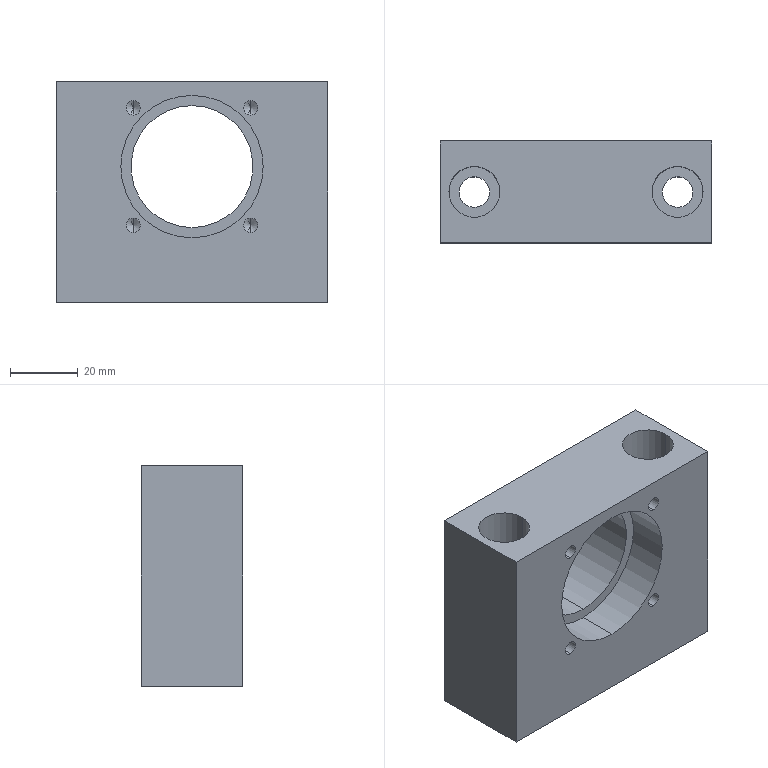Part | SolidWorks | features ICE 5, HoleWzd 4, Chamfer 1, Extrusion 1 | 1 solid | 37 faces | box 80 x 30 x 65 mm | volume 99631 mm3 | cylinder 20 | plane 9 | cone 8 | commonest cylinder face diameters 4.2 x8 9 x4 15 x4 36 x2 42 x2
STEP:
#1=CARTESIAN_POINT('',(17.324,-2.6,-7.724));
#2=VERTEX_POINT('',#1);
#3=CARTESIAN_POINT('',(17.324,-2.6,-11.924));
#4=VERTEX_POINT('',#3);
#5=CARTESIAN_POINT('',(17.324,-2.6,-9.824));
#6=DIRECTION('',(0.,-1.,0.));
#7=DIRECTION('',(0.,0.,-1.));
#8=AXIS2_PLACEMENT_3D('',#5,#6,#7);
#9=CIRCLE('',#8,2.1);
#10=EDGE_CURVE('',#2,#4,#9,.T.);
#11=ORIENTED_EDGE('',*,*,#10,.F.);
#12=CARTESIAN_POINT('',(17.324,-15.,-7.724));
#13=VERTEX_POINT('',#12);
#14=CARTESIAN_POINT('',(17.324,-15.,-7.724));
#15=DIRECTION('',(0.,-1.,0.));
#16=VECTOR('',#15,1000.);
#17=LINE('',#14,#16);
#18=EDGE_CURVE('',#2,#13,#17,.T.);
#19=ORIENTED_EDGE('',*,*,#18,.T.);
#20=CARTESIAN_POINT('',(17.324,-15.,-11.924));
#21=VERTEX_POINT('',#20);
#22=CARTESIAN_POINT('',(17.324,-15.,-9.824));
#23=DIRECTION('',(0.,-1.,0.));
#24=DIRECTION('',(0.,0.,-1.));
#25=AXIS2_PLACEMENT_3D('',#22,#23,#24);
#26=CIRCLE('',#25,2.1);
#27=EDGE_CURVE('',#13,#21,#26,.T.);
#28=ORIENTED_EDGE('',*,*,#27,.T.);
#29=CARTESIAN_POINT('',(17.324,-15.,-11.924));
#30=DIRECTION('',(0.,-1.,0.));
#31=VECTOR('',#30,1000.);
#32=LINE('',#29,#31);
#33=EDGE_CURVE('',#4,#21,#32,.T.);
#34=ORIENTED_EDGE('',*,*,#33,.F.);
#35=EDGE_LOOP('',(#11,#19,#28,#34));
#36=FACE_OUTER_BOUND('',#35,.T.);
#37=CARTESIAN_POINT('',(17.324,-15.,-9.824));
#38=DIRECTION('',(0.,-1.,0.));
#39=DIRECTION('',(0.,0.,-1.));
#40=AXIS2_PLACEMENT_3D('',#37,#38,#39);
#41=CYLINDRICAL_SURFACE('',#40,2.1);
#42=ADVANCED_FACE('',(#36),#41,.F.);
#43=CARTESIAN_POINT('',(17.324,-1.338,-9.824));
#44=VERTEX_POINT('',#43);
#45=CARTESIAN_POINT('',(17.324,-2.6,-11.924));
#46=DIRECTION('',(0.,-0.515,-0.8572));
#47=VECTOR('',#46,1000.);
#48=LINE('',#45,#47);
#49=EDGE_CURVE('',#44,#4,#48,.T.);
#50=ORIENTED_EDGE('',*,*,#49,.F.);
#51=CARTESIAN_POINT('',(17.324,-2.6,-7.724));
#52=DIRECTION('',(0.,-0.515,0.8572));
#53=VECTOR('',#52,1000.);
#54=LINE('',#51,#53);
#55=EDGE_CURVE('',#44,#2,#54,.T.);
#56=ORIENTED_EDGE('',*,*,#55,.T.);
#57=ORIENTED_EDGE('',*,*,#10,.T.);
#58=EDGE_LOOP('',(#50,#56,#57));
#59=FACE_OUTER_BOUND('',#58,.T.);
#60=CARTESIAN_POINT('',(17.324,-2.6,-9.824));
#61=DIRECTION('',(0.,-1.,0.));
#62=DIRECTION('',(0.,0.,-1.));
#63=AXIS2_PLACEMENT_3D('',#60,#61,#62);
#64=CONICAL_SURFACE('',#63,2.1,1.03);
#65=ADVANCED_FACE('',(#59),#64,.F.);
#66=CARTESIAN_POINT('',(-17.324,-2.6,-7.724));
#67=VERTEX_POINT('',#66);
#68=CARTESIAN_POINT('',(-17.324,-2.6,-11.924));
#69=VERTEX_POINT('',#68);
#70=CARTESIAN_POINT('',(-17.324,-2.6,-9.824));
#71=DIRECTION('',(0.,-1.,0.));
#72=DIRECTION('',(0.,0.,-1.));
#73=AXIS2_PLACEMENT_3D('',#70,#71,#72);
#74=CIRCLE('',#73,2.1);
#75=EDGE_CURVE('',#67,#69,#74,.T.);
#76=ORIENTED_EDGE('',*,*,#75,.F.);
#77=CARTESIAN_POINT('',(-17.324,-15.,-7.724));
#78=VERTEX_POINT('',#77);
#79=CARTESIAN_POINT('',(-17.324,-15.,-7.724));
#80=DIRECTION('',(0.,-1.,0.));
#81=VECTOR('',#80,1000.);
#82=LINE('',#79,#81);
#83=EDGE_CURVE('',#67,#78,#82,.T.);
#84=ORIENTED_EDGE('',*,*,#83,.T.);
#85=CARTESIAN_POINT('',(-17.324,-15.,-11.924));
#86=VERTEX_POINT('',#85);
#87=CARTESIAN_POINT('',(-17.324,-15.,-9.824));
#88=DIRECTION('',(0.,-1.,0.));
#89=DIRECTION('',(0.,0.,-1.));
#90=AXIS2_PLACEMENT_3D('',#87,#88,#89);
#91=CIRCLE('',#90,2.1);
#92=EDGE_CURVE('',#78,#86,#91,.T.);
#93=ORIENTED_EDGE('',*,*,#92,.T.);
#94=CARTESIAN_POINT('',(-17.324,-15.,-11.924));
#95=DIRECTION('',(0.,-1.,0.));
#96=VECTOR('',#95,1000.);
#97=LINE('',#94,#96);
#98=EDGE_CURVE('',#69,#86,#97,.T.);
#99=ORIENTED_EDGE('',*,*,#98,.F.);
#100=EDGE_LOOP('',(#76,#84,#93,#99));
#101=FACE_OUTER_BOUND('',#100,.T.);
#102=CARTESIAN_POINT('',(-17.324,-15.,-9.824));
#103=DIRECTION('',(0.,-1.,0.));
#104=DIRECTION('',(0.,0.,-1.));
#105=AXIS2_PLACEMENT_3D('',#102,#103,#104);
#106=CYLINDRICAL_SURFACE('',#105,2.1);
#107=ADVANCED_FACE('',(#101),#106,.F.);
#108=CARTESIAN_POINT('',(-17.324,-1.338,-9.824));
#109=VERTEX_POINT('',#108);
#110=CARTESIAN_POINT('',(-17.324,-2.6,-11.924));
#111=DIRECTION('',(0.,-0.515,-0.8572));
#112=VECTOR('',#111,1000.);
#113=LINE('',#110,#112);
#114=EDGE_CURVE('',#109,#69,#113,.T.);
#115=ORIENTED_EDGE('',*,*,#114,.F.);
#116=CARTESIAN_POINT('',(-17.324,-2.6,-7.724));
#117=DIRECTION('',(0.,-0.515,0.8572));
#118=VECTOR('',#117,1000.);
#119=LINE('',#116,#118);
#120=EDGE_CURVE('',#109,#67,#119,.T.);
#121=ORIENTED_EDGE('',*,*,#120,.T.);
#122=ORIENTED_EDGE('',*,*,#75,.T.);
#123=EDGE_LOOP('',(#115,#121,#122));
#124=FACE_OUTER_BOUND('',#123,.T.);
#125=CARTESIAN_POINT('',(-17.324,-2.6,-9.824));
#126=DIRECTION('',(0.,-1.,0.));
#127=DIRECTION('',(0.,0.,-1.));
#128=AXIS2_PLACEMENT_3D('',#125,#126,#127);
#129=CONICAL_SURFACE('',#128,2.1,1.03);
#130=ADVANCED_FACE('',(#124),#129,.F.);
#131=CARTESIAN_POINT('',(-17.324,-2.6,26.924));
#132=VERTEX_POINT('',#131);
#133=CARTESIAN_POINT('',(-17.324,-2.6,22.724));
#134=VERTEX_POINT('',#133);
#135=CARTESIAN_POINT('',(-17.324,-2.6,24.824));
#136=DIRECTION('',(0.,-1.,0.));
#137=DIRECTION('',(0.,0.,-1.));
#138=AXIS2_PLACEMENT_3D('',#135,#136,#137);
#139=CIRCLE('',#138,2.1);
#140=EDGE_CURVE('',#132,#134,#139,.T.);
#141=ORIENTED_EDGE('',*,*,#140,.F.);
#142=CARTESIAN_POINT('',(-17.324,-15.,26.924));
#143=VERTEX_POINT('',#142);
#144=CARTESIAN_POINT('',(-17.324,-15.,26.924));
#145=DIRECTION('',(0.,-1.,0.));
#146=VECTOR('',#145,1000.);
#147=LINE('',#144,#146);
#148=EDGE_CURVE('',#132,#143,#147,.T.);
#149=ORIENTED_EDGE('',*,*,#148,.T.);
#150=CARTESIAN_POINT('',(-17.324,-15.,22.724));
#151=VERTEX_POINT('',#150);
#152=CARTESIAN_POINT('',(-17.324,-15.,24.824));
#153=DIRECTION('',(0.,-1.,0.));
#154=DIRECTION('',(0.,0.,-1.));
#155=AXIS2_PLACEMENT_3D('',#152,#153,#154);
#156=CIRCLE('',#155,2.1);
#157=EDGE_CURVE('',#143,#151,#156,.T.);
#158=ORIENTED_EDGE('',*,*,#157,.T.);
#159=CARTESIAN_POINT('',(-17.324,-15.,22.724));
#160=DIRECTION('',(0.,-1.,0.));
#161=VECTOR('',#160,1000.);
#162=LINE('',#159,#161);
#163=EDGE_CURVE('',#134,#151,#162,.T.);
#164=ORIENTED_EDGE('',*,*,#163,.F.);
#165=EDGE_LOOP('',(#141,#149,#158,#164));
#166=FACE_OUTER_BOUND('',#165,.T.);
#167=CARTESIAN_POINT('',(-17.324,-15.,24.824));
#168=DIRECTION('',(0.,-1.,0.));
#169=DIRECTION('',(0.,0.,-1.));
#170=AXIS2_PLACEMENT_3D('',#167,#168,#169);
#171=CYLINDRICAL_SURFACE('',#170,2.1);
#172=ADVANCED_FACE('',(#166),#171,.F.);
#173=CARTESIAN_POINT('',(-17.324,-1.338,24.824));
#174=VERTEX_POINT('',#173);
#175=CARTESIAN_POINT('',(-17.324,-2.6,22.724));
#176=DIRECTION('',(0.,-0.515,-0.8572));
#177=VECTOR('',#176,1000.);
#178=LINE('',#175,#177);
#179=EDGE_CURVE('',#174,#134,#178,.T.);
#180=ORIENTED_EDGE('',*,*,#179,.F.);
#181=CARTESIAN_POINT('',(-17.324,-2.6,26.924));
#182=DIRECTION('',(0.,-0.515,0.8572));
#183=VECTOR('',#182,1000.);
#184=LINE('',#181,#183);
#185=EDGE_CURVE('',#174,#132,#184,.T.);
#186=ORIENTED_EDGE('',*,*,#185,.T.);
#187=ORIENTED_EDGE('',*,*,#140,.T.);
#188=EDGE_LOOP('',(#180,#186,#187));
#189=FACE_OUTER_BOUND('',#188,.T.);
#190=CARTESIAN_POINT('',(-17.324,-2.6,24.824));
#191=DIRECTION('',(0.,-1.,0.));
#192=DIRECTION('',(0.,0.,-1.));
#193=AXIS2_PLACEMENT_3D('',#190,#191,#192);
#194=CONICAL_SURFACE('',#193,2.1,1.03);
#195=ADVANCED_FACE('',(#189),#194,.F.);
#196=CARTESIAN_POINT('',(17.324,-2.6,26.924));
#197=VERTEX_POINT('',#196);
#198=CARTESIAN_POINT('',(17.324,-2.6,22.724));
#199=VERTEX_POINT('',#198);
#200=CARTESIAN_POINT('',(17.324,-2.6,24.824));
#201=DIRECTION('',(0.,-1.,0.));
#202=DIRECTION('',(0.,0.,-1.));
#203=AXIS2_PLACEMENT_3D('',#200,#201,#202);
#204=CIRCLE('',#203,2.1);
#205=EDGE_CURVE('',#197,#199,#204,.T.);
#206=ORIENTED_EDGE('',*,*,#205,.F.);
#207=CARTESIAN_POINT('',(17.324,-15.,26.924));
#208=VERTEX_POINT('',#207);
#209=CARTESIAN_POINT('',(17.324,-15.,26.924));
#210=DIRECTION('',(0.,-1.,0.));
#211=VECTOR('',#210,1000.);
#212=LINE('',#209,#211);
#213=EDGE_CURVE('',#197,#208,#212,.T.);
#214=ORIENTED_EDGE('',*,*,#213,.T.);
#215=CARTESIAN_POINT('',(17.324,-15.,22.724));
#216=VERTEX_POINT('',#215);
#217=CARTESIAN_POINT('',(17.324,-15.,24.824));
#218=DIRECTION('',(0.,-1.,0.));
#219=DIRECTION('',(0.,0.,-1.));
#220=AXIS2_PLACEMENT_3D('',#217,#218,#219);
#221=CIRCLE('',#220,2.1);
#222=EDGE_CURVE('',#208,#216,#221,.T.);
#223=ORIENTED_EDGE('',*,*,#222,.T.);
#224=CARTESIAN_POINT('',(17.324,-15.,22.724));
#225=DIRECTION('',(0.,-1.,0.));
#226=VECTOR('',#225,1000.);
#227=LINE('',#224,#226);
#228=EDGE_CURVE('',#199,#216,#227,.T.);
#229=ORIENTED_EDGE('',*,*,#228,.F.);
#230=EDGE_LOOP('',(#206,#214,#223,#229));
#231=FACE_OUTER_BOUND('',#230,.T.);
#232=CARTESIAN_POINT('',(17.324,-15.,24.824));
#233=DIRECTION('',(0.,-1.,0.));
#234=DIRECTION('',(0.,0.,-1.));
#235=AXIS2_PLACEMENT_3D('',#232,#233,#234);
#236=CYLINDRICAL_SURFACE('',#235,2.1);
#237=ADVANCED_FACE('',(#231),#236,.F.);
#238=CARTESIAN_POINT('',(17.324,-1.338,24.824));
#239=VERTEX_POINT('',#238);
#240=CARTESIAN_POINT('',(17.324,-2.6,22.724));
#241=DIRECTION('',(0.,-0.515,-0.8572));
#242=VECTOR('',#241,1000.);
#243=LINE('',#240,#242);
#244=EDGE_CURVE('',#239,#199,#243,.T.);
#245=ORIENTED_EDGE('',*,*,#244,.F.);
#246=CARTESIAN_POINT('',(17.324,-2.6,26.924));
#247=DIRECTION('',(0.,-0.515,0.8572));
#248=VECTOR('',#247,1000.);
#249=LINE('',#246,#248);
#250=EDGE_CURVE('',#239,#197,#249,.T.);
#251=ORIENTED_EDGE('',*,*,#250,.T.);
#252=ORIENTED_EDGE('',*,*,#205,.T.);
#253=EDGE_LOOP('',(#245,#251,#252));
#254=FACE_OUTER_BOUND('',#253,.T.);
#255=CARTESIAN_POINT('',(17.324,-2.6,24.824));
#256=DIRECTION('',(0.,-1.,0.));
#257=DIRECTION('',(0.,0.,-1.));
#258=AXIS2_PLACEMENT_3D('',#255,#256,#257);
#259=CONICAL_SURFACE('',#258,2.1,1.03);
#260=ADVANCED_FACE('',(#254),#259,.F.);
#261=CARTESIAN_POINT('',(22.5,0.,-22.5));
#262=VERTEX_POINT('',#261);
#263=CARTESIAN_POINT('',(37.5,0.,-22.5));
#264=VERTEX_POINT('',#263);
#265=CARTESIAN_POINT('',(30.,0.,-22.5));
#266=DIRECTION('',(0.,0.,1.));
#267=DIRECTION('',(1.,0.,0.));
#268=AXIS2_PLACEMENT_3D('',#265,#266,#267);
#269=CIRCLE('',#268,7.5);
#270=EDGE_CURVE('',#262,#264,#269,.T.);
#271=ORIENTED_EDGE('',*,*,#270,.F.);
#272=CARTESIAN_POINT('',(22.5,0.,32.5));
#273=VERTEX_POINT('',#272);
#274=CARTESIAN_POINT('',(22.5,0.,32.5));
#275=DIRECTION('',(0.,0.,1.));
#276=VECTOR('',#275,1000.);
#277=LINE('',#274,#276);
#278=EDGE_CURVE('',#262,#273,#277,.T.);
#279=ORIENTED_EDGE('',*,*,#278,.T.);
#280=CARTESIAN_POINT('',(37.5,0.,32.5));
#281=VERTEX_POINT('',#280);
#282=CARTESIAN_POINT('',(30.,0.,32.5));
#283=DIRECTION('',(0.,0.,1.));
#284=DIRECTION('',(1.,0.,0.));
#285=AXIS2_PLACEMENT_3D('',#282,#283,#284);
#286=CIRCLE('',#285,7.5);
#287=EDGE_CURVE('',#273,#281,#286,.T.);
#288=ORIENTED_EDGE('',*,*,#287,.T.);
#289=CARTESIAN_POINT('',(37.5,0.,32.5));
#290=DIRECTION('',(0.,0.,1.));
#291=VECTOR('',#290,1000.);
#292=LINE('',#289,#291);
#293=EDGE_CURVE('',#264,#281,#292,.T.);
#294=ORIENTED_EDGE('',*,*,#293,.F.);
#295=EDGE_LOOP('',(#271,#279,#288,#294));
#296=FACE_OUTER_BOUND('',#295,.T.);
#297=CARTESIAN_POINT('',(30.,0.,32.5));
#298=DIRECTION('',(0.,0.,1.));
#299=DIRECTION('',(1.,0.,0.));
#300=AXIS2_PLACEMENT_3D('',#297,#298,#299);
#301=CYLINDRICAL_SURFACE('',#300,7.5);
#302=ADVANCED_FACE('',(#296),#301,.F.);
#303=CARTESIAN_POINT('',(25.5,0.,-32.5));
#304=VERTEX_POINT('',#303);
#305=CARTESIAN_POINT('',(34.5,0.,-32.5));
#306=VERTEX_POINT('',#305);
#307=CARTESIAN_POINT('',(30.,0.,-32.5));
#308=DIRECTION('',(0.,0.,1.));
#309=DIRECTION('',(1.,0.,0.));
#310=AXIS2_PLACEMENT_3D('',#307,#308,#309);
#311=CIRCLE('',#310,4.5);
#312=EDGE_CURVE('',#304,#306,#311,.T.);
#313=ORIENTED_EDGE('',*,*,#312,.F.);
#314=CARTESIAN_POINT('',(25.5,0.,-22.5));
#315=VERTEX_POINT('',#314);
#316=CARTESIAN_POINT('',(25.5,0.,32.5));
#317=DIRECTION('',(0.,0.,1.));
#318=VECTOR('',#317,1000.);
#319=LINE('',#316,#318);
#320=EDGE_CURVE('',#304,#315,#319,.T.);
#321=ORIENTED_EDGE('',*,*,#320,.T.);
#322=CARTESIAN_POINT('',(34.5,0.,-22.5));
#323=VERTEX_POINT('',#322);
#324=CARTESIAN_POINT('',(30.,0.,-22.5));
#325=DIRECTION('',(0.,0.,1.));
#326=DIRECTION('',(1.,0.,0.));
#327=AXIS2_PLACEMENT_3D('',#324,#325,#326);
#328=CIRCLE('',#327,4.5);
#329=EDGE_CURVE('',#315,#323,#328,.T.);
#330=ORIENTED_EDGE('',*,*,#329,.T.);
#331=CARTESIAN_POINT('',(34.5,0.,32.5));
#332=DIRECTION('',(0.,0.,1.));
#333=VECTOR('',#332,1000.);
#334=LINE('',#331,#333);
#335=EDGE_CURVE('',#306,#323,#334,.T.);
#336=ORIENTED_EDGE('',*,*,#335,.F.);
#337=EDGE_LOOP('',(#313,#321,#330,#336));
#338=FACE_OUTER_BOUND('',#337,.T.);
#339=CARTESIAN_POINT('',(30.,0.,32.5));
#340=DIRECTION('',(0.,0.,1.));
#341=DIRECTION('',(1.,0.,0.));
#342=AXIS2_PLACEMENT_3D('',#339,#340,#341);
#343=CYLINDRICAL_SURFACE('',#342,4.5);
#344=ADVANCED_FACE('',(#338),#343,.F.);
#345=CARTESIAN_POINT('',(-37.5,0.,-22.5));
#346=VERTEX_POINT('',#345);
#347=CARTESIAN_POINT('',(-22.5,0.,-22.5));
#348=VERTEX_POINT('',#347);
#349=CARTESIAN_POINT('',(-30.,0.,-22.5));
#350=DIRECTION('',(0.,0.,1.));
#351=DIRECTION('',(1.,0.,0.));
#352=AXIS2_PLACEMENT_3D('',#349,#350,#351);
#353=CIRCLE('',#352,7.5);
#354=EDGE_CURVE('',#346,#348,#353,.T.);
#355=ORIENTED_EDGE('',*,*,#354,.F.);
#356=CARTESIAN_POINT('',(-37.5,0.,32.5));
#357=VERTEX_POINT('',#356);
#358=CARTESIAN_POINT('',(-37.5,0.,32.5));
#359=DIRECTION('',(0.,0.,1.));
#360=VECTOR('',#359,1000.);
#361=LINE('',#358,#360);
#362=EDGE_CURVE('',#346,#357,#361,.T.);
#363=ORIENTED_EDGE('',*,*,#362,.T.);
#364=CARTESIAN_POINT('',(-22.5,0.,32.5));
#365=VERTEX_POINT('',#364);
#366=CARTESIAN_POINT('',(-30.,0.,32.5));
#367=DIRECTION('',(0.,0.,1.));
#368=DIRECTION('',(1.,0.,0.));
#369=AXIS2_PLACEMENT_3D('',#366,#367,#368);
#370=CIRCLE('',#369,7.5);
#371=EDGE_CURVE('',#357,#365,#370,.T.);
#372=ORIENTED_EDGE('',*,*,#371,.T.);
#373=CARTESIAN_POINT('',(-22.5,0.,32.5));
#374=DIRECTION('',(0.,0.,1.));
#375=VECTOR('',#374,1000.);
#376=LINE('',#373,#375);
#377=EDGE_CURVE('',#348,#365,#376,.T.);
#378=ORIENTED_EDGE('',*,*,#377,.F.);
#379=EDGE_LOOP('',(#355,#363,#372,#378));
#380=FACE_OUTER_BOUND('',#379,.T.);
#381=CARTESIAN_POINT('',(-30.,0.,32.5));
#382=DIRECTION('',(0.,0.,1.));
#383=DIRECTION('',(1.,0.,0.));
#384=AXIS2_PLACEMENT_3D('',#381,#382,#383);
#385=CYLINDRICAL_SURFACE('',#384,7.5);
#386=ADVANCED_FACE('',(#380),#385,.F.);
#387=CARTESIAN_POINT('',(-34.5,0.,-32.5));
#388=VERTEX_POINT('',#387);
#389=CARTESIAN_POINT('',(-25.5,0.,-32.5));
#390=VERTEX_POINT('',#389);
#391=CARTESIAN_POINT('',(-30.,0.,-32.5));
#392=DIRECTION('',(0.,0.,1.));
#393=DIRECTION('',(1.,0.,0.));
#394=AXIS2_PLACEMENT_3D('',#391,#392,#393);
#395=CIRCLE('',#394,4.5);
#396=EDGE_CURVE('',#388,#390,#395,.T.);
#397=ORIENTED_EDGE('',*,*,#396,.F.);
#398=CARTESIAN_POINT('',(-34.5,0.,-22.5));
#399=VERTEX_POINT('',#398);
#400=CARTESIAN_POINT('',(-34.5,0.,32.5));
#401=DIRECTION('',(0.,0.,1.));
#402=VECTOR('',#401,1000.);
#403=LINE('',#400,#402);
#404=EDGE_CURVE('',#388,#399,#403,.T.);
#405=ORIENTED_EDGE('',*,*,#404,.T.);
#406=CARTESIAN_POINT('',(-25.5,0.,-22.5));
#407=VERTEX_POINT('',#406);
#408=CARTESIAN_POINT('',(-30.,0.,-22.5));
#409=DIRECTION('',(0.,0.,1.));
#410=DIRECTION('',(1.,0.,0.));
#411=AXIS2_PLACEMENT_3D('',#408,#409,#410);
#412=CIRCLE('',#411,4.5);
#413=EDGE_CURVE('',#399,#407,#412,.T.);
#414=ORIENTED_EDGE('',*,*,#413,.T.);
#415=CARTESIAN_POINT('',(-25.5,0.,32.5));
#416=DIRECTION('',(0.,0.,1.));
#417=VECTOR('',#416,1000.);
#418=LINE('',#415,#417);
#419=EDGE_CURVE('',#390,#407,#418,.T.);
#420=ORIENTED_EDGE('',*,*,#419,.F.);
#421=EDGE_LOOP('',(#397,#405,#414,#420));
#422=FACE_OUTER_BOUND('',#421,.T.);
#423=CARTESIAN_POINT('',(-30.,0.,32.5));
#424=DIRECTION('',(0.,0.,1.));
#425=DIRECTION('',(1.,0.,0.));
#426=AXIS2_PLACEMENT_3D('',#423,#424,#425);
#427=CYLINDRICAL_SURFACE('',#426,4.5);
#428=ADVANCED_FACE('',(#422),#427,.F.);
#429=CARTESIAN_POINT('',(0.,15.,25.5));
#430=VERTEX_POINT('',#429);
#431=CARTESIAN_POINT('',(0.,15.,-10.5));
#432=VERTEX_POINT('',#431);
#433=CARTESIAN_POINT('',(0.,15.,7.5));
#434=DIRECTION('',(0.,-1.,0.));
#435=DIRECTION('',(0.,0.,-1.));
#436=AXIS2_PLACEMENT_3D('',#433,#434,#435);
#437=CIRCLE('',#436,18.);
#438=EDGE_CURVE('',#430,#432,#437,.T.);
#439=ORIENTED_EDGE('',*,*,#438,.F.);
#440=CARTESIAN_POINT('',(0.,-3.,25.5));
#441=VERTEX_POINT('',#440);
#442=CARTESIAN_POINT('',(0.,15.,25.5));
#443=DIRECTION('',(0.,-1.,0.));
#444=VECTOR('',#443,1000.);
#445=LINE('',#442,#444);
#446=EDGE_CURVE('',#430,#441,#445,.T.);
#447=ORIENTED_EDGE('',*,*,#446,.T.);
#448=CARTESIAN_POINT('',(0.,-3.,-10.5));
#449=VERTEX_POINT('',#448);
#450=CARTESIAN_POINT('',(0.,-3.,7.5));
#451=DIRECTION('',(0.,-1.,0.));
#452=DIRECTION('',(0.,0.,-1.));
#453=AXIS2_PLACEMENT_3D('',#450,#451,#452);
#454=CIRCLE('',#453,18.);
#455=EDGE_CURVE('',#441,#449,#454,.T.);
#456=ORIENTED_EDGE('',*,*,#455,.T.);
#457=CARTESIAN_POINT('',(0.,15.,-10.5));
#458=DIRECTION('',(0.,-1.,0.));
#459=VECTOR('',#458,1000.);
#460=LINE('',#457,#459);
#461=EDGE_CURVE('',#432,#449,#460,.T.);
#462=ORIENTED_EDGE('',*,*,#461,.F.);
#463=EDGE_LOOP('',(#439,#447,#456,#462));
#464=FACE_OUTER_BOUND('',#463,.T.);
#465=CARTESIAN_POINT('',(0.,15.,7.5));
#466=DIRECTION('',(0.,-1.,0.));
#467=DIRECTION('',(0.,0.,-1.));
#468=AXIS2_PLACEMENT_3D('',#465,#466,#467);
#469=CYLINDRICAL_SURFACE('',#468,18.);
#470=ADVANCED_FACE('',(#464),#469,.F.);
#471=CARTESIAN_POINT('',(0.,-3.,-13.5));
#472=VERTEX_POINT('',#471);
#473=CARTESIAN_POINT('',(0.,-3.,28.5));
#474=VERTEX_POINT('',#473);
#475=CARTESIAN_POINT('',(0.,-3.,7.5));
#476=DIRECTION('',(0.,1.,0.));
#477=DIRECTION('',(0.,0.,1.));
#478=AXIS2_PLACEMENT_3D('',#475,#476,#477);
#479=CIRCLE('',#478,21.);
#480=EDGE_CURVE('',#472,#474,#479,.T.);
#481=ORIENTED_EDGE('',*,*,#480,.T.);
#482=CARTESIAN_POINT('',(0.,-15.,28.5));
#483=VERTEX_POINT('',#482);
#484=CARTESIAN_POINT('',(0.,-3.,28.5));
#485=DIRECTION('',(0.,-1.,0.));
#486=VECTOR('',#485,1000.);
#487=LINE('',#484,#486);
#488=EDGE_CURVE('',#474,#483,#487,.T.);
#489=ORIENTED_EDGE('',*,*,#488,.T.);
#490=CARTESIAN_POINT('',(0.,-15.,-13.5));
#491=VERTEX_POINT('',#490);
#492=CARTESIAN_POINT('',(0.,-15.,7.5));
#493=DIRECTION('',(0.,1.,0.));
#494=DIRECTION('',(0.,0.,1.));
#495=AXIS2_PLACEMENT_3D('',#492,#493,#494);
#496=CIRCLE('',#495,21.);
#497=EDGE_CURVE('',#491,#483,#496,.T.);
#498=ORIENTED_EDGE('',*,*,#497,.F.);
#499=CARTESIAN_POINT('',(0.,-3.,-13.5));
#500=DIRECTION('',(0.,-1.,0.));
#501=VECTOR('',#500,1000.);
#502=LINE('',#499,#501);
#503=EDGE_CURVE('',#472,#491,#502,.T.);
#504=ORIENTED_EDGE('',*,*,#503,.F.);
#505=EDGE_LOOP('',(#481,#489,#498,#504));
#506=FACE_OUTER_BOUND('',#505,.T.);
#507=CARTESIAN_POINT('',(0.,-3.,7.5));
#508=DIRECTION('',(0.,-1.,0.));
#509=DIRECTION('',(0.,0.,-1.));
#510=AXIS2_PLACEMENT_3D('',#507,#508,#509);
#511=CYLINDRICAL_SURFACE('',#510,21.);
#512=ADVANCED_FACE('',(#506),#511,.F.);
#513=CARTESIAN_POINT('',(30.,0.,32.5));
#514=DIRECTION('',(0.,0.,1.));
#515=DIRECTION('',(1.,0.,0.));
#516=AXIS2_PLACEMENT_3D('',#513,#514,#515);
#517=CIRCLE('',#516,7.5);
#518=EDGE_CURVE('',#281,#273,#517,.T.);
#519=ORIENTED_EDGE('',*,*,#518,.F.);
#520=ORIENTED_EDGE('',*,*,#287,.F.);
#521=EDGE_LOOP('',(#519,#520));
#522=FACE_BOUND('',#521,.T.);
#523=CARTESIAN_POINT('',(-30.,0.,32.5));
#524=DIRECTION('',(0.,0.,1.));
#525=DIRECTION('',(1.,0.,0.));
#526=AXIS2_PLACEMENT_3D('',#523,#524,#525);
#527=CIRCLE('',#526,7.5);
#528=EDGE_CURVE('',#365,#357,#527,.T.);
#529=ORIENTED_EDGE('',*,*,#528,.F.);
#530=ORIENTED_EDGE('',*,*,#371,.F.);
#531=EDGE_LOOP('',(#529,#530));
#532=FACE_BOUND('',#531,.T.);
#533=CARTESIAN_POINT('',(-40.,-15.,32.5));
#534=VERTEX_POINT('',#533);
#535=CARTESIAN_POINT('',(40.,-15.,32.5));
#536=VERTEX_POINT('',#535);
#537=CARTESIAN_POINT('',(-225.,-15.,32.5));
#538=DIRECTION('',(1.,0.,0.));
#539=VECTOR('',#538,1000.);
#540=LINE('',#537,#539);
#541=EDGE_CURVE('',#534,#536,#540,.T.);
#542=ORIENTED_EDGE('',*,*,#541,.T.);
#543=CARTESIAN_POINT('',(40.,15.,32.5));
#544=VERTEX_POINT('',#543);
#545=CARTESIAN_POINT('',(40.,15.,32.5));
#546=DIRECTION('',(0.,1.,0.));
#547=VECTOR('',#546,1000.);
#548=LINE('',#545,#547);
#549=EDGE_CURVE('',#536,#544,#548,.T.);
#550=ORIENTED_EDGE('',*,*,#549,.T.);
#551=CARTESIAN_POINT('',(-40.,15.,32.5));
#552=VERTEX_POINT('',#551);
#553=CARTESIAN_POINT('',(-225.,15.,32.5));
#554=DIRECTION('',(1.,0.,0.));
#555=VECTOR('',#554,1000.);
#556=LINE('',#553,#555);
#557=EDGE_CURVE('',#552,#544,#556,.T.);
#558=ORIENTED_EDGE('',*,*,#557,.F.);
#559=CARTESIAN_POINT('',(-40.,15.,32.5));
#560=DIRECTION('',(0.,-1.,0.));
#561=VECTOR('',#560,1000.);
#562=LINE('',#559,#561);
#563=EDGE_CURVE('',#552,#534,#562,.T.);
#564=ORIENTED_EDGE('',*,*,#563,.T.);
#565=EDGE_LOOP('',(#542,#550,#558,#564));
#566=FACE_OUTER_BOUND('',#565,.T.);
#567=CARTESIAN_POINT('',(-225.,15.,32.5));
#568=DIRECTION('',(0.,0.,-1.));
#569=DIRECTION('',(-1.,0.,0.));
#570=AXIS2_PLACEMENT_3D('',#567,#568,#569);
#571=PLANE('',#570);
#572=ADVANCED_FACE('',(#522,#532,#566),#571,.F.);
#573=CARTESIAN_POINT('',(30.,0.,-32.5));
#574=DIRECTION('',(0.,0.,1.));
#575=DIRECTION('',(1.,0.,0.));
#576=AXIS2_PLACEMENT_3D('',#573,#574,#575);
#577=CIRCLE('',#576,4.5);
#578=EDGE_CURVE('',#306,#304,#577,.T.);
#579=ORIENTED_EDGE('',*,*,#578,.T.);
#580=ORIENTED_EDGE('',*,*,#312,.T.);
#581=EDGE_LOOP('',(#579,#580));
#582=FACE_BOUND('',#581,.T.);
#583=CARTESIAN_POINT('',(-30.,0.,-32.5));
#584=DIRECTION('',(0.,0.,1.));
#585=DIRECTION('',(1.,0.,0.));
#586=AXIS2_PLACEMENT_3D('',#583,#584,#585);
#587=CIRCLE('',#586,4.5);
#588=EDGE_CURVE('',#390,#388,#587,.T.);
#589=ORIENTED_EDGE('',*,*,#588,.T.);
#590=ORIENTED_EDGE('',*,*,#396,.T.);
#591=EDGE_LOOP('',(#589,#590));
#592=FACE_BOUND('',#591,.T.);
#593=CARTESIAN_POINT('',(40.,15.,-32.5));
#594=VERTEX_POINT('',#593);
#595=CARTESIAN_POINT('',(-40.,15.,-32.5));
#596=VERTEX_POINT('',#595);
#597=CARTESIAN_POINT('',(-225.,15.,-32.5));
#598=DIRECTION('',(-1.,0.,0.));
#599=VECTOR('',#598,1000.);
#600=LINE('',#597,#599);
#601=EDGE_CURVE('',#594,#596,#600,.T.);
#602=ORIENTED_EDGE('',*,*,#601,.F.);
#603=CARTESIAN_POINT('',(40.,-15.,-32.5));
#604=VERTEX_POINT('',#603);
#605=CARTESIAN_POINT('',(40.,15.,-32.5));
#606=DIRECTION('',(0.,-1.,0.));
#607=VECTOR('',#606,1000.);
#608=LINE('',#605,#607);
#609=EDGE_CURVE('',#594,#604,#608,.T.);
#610=ORIENTED_EDGE('',*,*,#609,.T.);
#611=CARTESIAN_POINT('',(-40.,-15.,-32.5));
#612=VERTEX_POINT('',#611);
#613=CARTESIAN_POINT('',(-225.,-15.,-32.5));
#614=DIRECTION('',(-1.,0.,0.));
#615=VECTOR('',#614,1000.);
#616=LINE('',#613,#615);
#617=EDGE_CURVE('',#604,#612,#616,.T.);
#618=ORIENTED_EDGE('',*,*,#617,.T.);
#619=CARTESIAN_POINT('',(-40.,15.,-32.5));
#620=DIRECTION('',(0.,1.,0.));
#621=VECTOR('',#620,1000.);
#622=LINE('',#619,#621);
#623=EDGE_CURVE('',#612,#596,#622,.T.);
#624=ORIENTED_EDGE('',*,*,#623,.T.);
#625=EDGE_LOOP('',(#602,#610,#618,#624));
#626=FACE_OUTER_BOUND('',#625,.T.);
#627=CARTESIAN_POINT('',(-225.,15.,-32.5));
#628=DIRECTION('',(0.,0.,1.));
#629=DIRECTION('',(1.,0.,0.));
#630=AXIS2_PLACEMENT_3D('',#627,#628,#629);
#631=PLANE('',#630);
#632=ADVANCED_FACE('',(#582,#592,#626),#631,.F.);
#633=CARTESIAN_POINT('',(0.,15.,7.5));
#634=DIRECTION('',(0.,-1.,0.));
#635=DIRECTION('',(0.,0.,-1.));
#636=AXIS2_PLACEMENT_3D('',#633,#634,#635);
#637=CIRCLE('',#636,18.);
#638=EDGE_CURVE('',#432,#430,#637,.T.);
#639=ORIENTED_EDGE('',*,*,#638,.T.);
#640=ORIENTED_EDGE('',*,*,#438,.T.);
#641=EDGE_LOOP('',(#639,#640));
#642=FACE_BOUND('',#641,.T.);
#643=ORIENTED_EDGE('',*,*,#557,.T.);
#644=CARTESIAN_POINT('',(40.,15.,-66.164));
#645=DIRECTION('',(0.,0.,-1.));
#646=VECTOR('',#645,1000.);
#647=LINE('',#644,#646);
#648=EDGE_CURVE('',#544,#594,#647,.T.);
#649=ORIENTED_EDGE('',*,*,#648,.T.);
#650=ORIENTED_EDGE('',*,*,#601,.T.);
#651=CARTESIAN_POINT('',(-40.,15.,-66.164));
#652=DIRECTION('',(0.,0.,1.));
#653=VECTOR('',#652,1000.);
#654=LINE('',#651,#653);
#655=EDGE_CURVE('',#596,#552,#654,.T.);
#656=ORIENTED_EDGE('',*,*,#655,.T.);
#657=EDGE_LOOP('',(#643,#649,#650,#656));
#658=FACE_OUTER_BOUND('',#657,.T.);
#659=CARTESIAN_POINT('',(0.,15.,0.));
#660=DIRECTION('',(0.,-1.,0.));
#661=DIRECTION('',(0.,0.,-1.));
#662=AXIS2_PLACEMENT_3D('',#659,#660,#661);
#663=PLANE('',#662);
#664=ADVANCED_FACE('',(#642,#658),#663,.F.);
#665=CARTESIAN_POINT('',(40.,-15.,-66.164));
#666=DIRECTION('',(0.,0.,-1.));
#667=VECTOR('',#666,1000.);
#668=LINE('',#665,#667);
#669=EDGE_CURVE('',#536,#604,#668,.T.);
#670=ORIENTED_EDGE('',*,*,#669,.F.);
#671=ORIENTED_EDGE('',*,*,#541,.F.);
#672=CARTESIAN_POINT('',(-40.,-15.,-66.164));
#673=DIRECTION('',(0.,0.,1.));
#674=VECTOR('',#673,1000.);
#675=LINE('',#672,#674);
#676=EDGE_CURVE('',#612,#534,#675,.T.);
#677=ORIENTED_EDGE('',*,*,#676,.F.);
#678=ORIENTED_EDGE('',*,*,#617,.F.);
#679=EDGE_LOOP('',(#670,#671,#677,#678));
#680=FACE_OUTER_BOUND('',#679,.T.);
#681=CARTESIAN_POINT('',(17.324,-15.,-9.824));
#682=DIRECTION('',(0.,-1.,0.));
#683=DIRECTION('',(0.,0.,-1.));
#684=AXIS2_PLACEMENT_3D('',#681,#682,#683);
#685=CIRCLE('',#684,2.1);
#686=EDGE_CURVE('',#21,#13,#685,.T.);
#687=ORIENTED_EDGE('',*,*,#686,.F.);
#688=ORIENTED_EDGE('',*,*,#27,.F.);
#689=EDGE_LOOP('',(#687,#688));
#690=FACE_BOUND('',#689,.T.);
#691=CARTESIAN_POINT('',(-17.324,-15.,-9.824));
#692=DIRECTION('',(0.,-1.,0.));
#693=DIRECTION('',(0.,0.,-1.));
#694=AXIS2_PLACEMENT_3D('',#691,#692,#693);
#695=CIRCLE('',#694,2.1);
#696=EDGE_CURVE('',#86,#78,#695,.T.);
#697=ORIENTED_EDGE('',*,*,#696,.F.);
#698=ORIENTED_EDGE('',*,*,#92,.F.);
#699=EDGE_LOOP('',(#697,#698));
#700=FACE_BOUND('',#699,.T.);
#701=CARTESIAN_POINT('',(-17.324,-15.,24.824));
#702=DIRECTION('',(0.,-1.,0.));
#703=DIRECTION('',(0.,0.,-1.));
#704=AXIS2_PLACEMENT_3D('',#701,#702,#703);
#705=CIRCLE('',#704,2.1);
#706=EDGE_CURVE('',#151,#143,#705,.T.);
#707=ORIENTED_EDGE('',*,*,#706,.F.);
#708=ORIENTED_EDGE('',*,*,#157,.F.);
#709=EDGE_LOOP('',(#707,#708));
#710=FACE_BOUND('',#709,.T.);
#711=CARTESIAN_POINT('',(17.324,-15.,24.824));
#712=DIRECTION('',(0.,-1.,0.));
#713=DIRECTION('',(0.,0.,-1.));
#714=AXIS2_PLACEMENT_3D('',#711,#712,#713);
#715=CIRCLE('',#714,2.1);
#716=EDGE_CURVE('',#216,#208,#715,.T.);
#717=ORIENTED_EDGE('',*,*,#716,.F.);
#718=ORIENTED_EDGE('',*,*,#222,.F.);
#719=EDGE_LOOP('',(#717,#718));
#720=FACE_BOUND('',#719,.T.);
#721=ORIENTED_EDGE('',*,*,#497,.T.);
#722=CARTESIAN_POINT('',(0.,-15.,7.5));
#723=DIRECTION('',(0.,1.,0.));
#724=DIRECTION('',(0.,0.,1.));
#725=AXIS2_PLACEMENT_3D('',#722,#723,#724);
#726=CIRCLE('',#725,21.);
#727=EDGE_CURVE('',#483,#491,#726,.T.);
#728=ORIENTED_EDGE('',*,*,#727,.T.);
#729=EDGE_LOOP('',(#721,#728));
#730=FACE_BOUND('',#729,.T.);
#731=CARTESIAN_POINT('',(0.,-15.,0.));
#732=DIRECTION('',(0.,-1.,0.));
#733=DIRECTION('',(0.,0.,-1.));
#734=AXIS2_PLACEMENT_3D('',#731,#732,#733);
#735=PLANE('',#734);
#736=ADVANCED_FACE('',(#680,#690,#700,#710,#720,#730),#735,.T.);
#737=ORIENTED_EDGE('',*,*,#488,.F.);
#738=CARTESIAN_POINT('',(0.,-3.,7.5));
#739=DIRECTION('',(0.,1.,0.));
#740=DIRECTION('',(0.,0.,1.));
#741=AXIS2_PLACEMENT_3D('',#738,#739,#740);
#742=CIRCLE('',#741,21.);
#743=EDGE_CURVE('',#474,#472,#742,.T.);
#744=ORIENTED_EDGE('',*,*,#743,.T.);
#745=ORIENTED_EDGE('',*,*,#503,.T.);
#746=ORIENTED_EDGE('',*,*,#727,.F.);
#747=EDGE_LOOP('',(#737,#744,#745,#746));
#748=FACE_OUTER_BOUND('',#747,.T.);
#749=CARTESIAN_POINT('',(0.,-3.,7.5));
#750=DIRECTION('',(0.,-1.,0.));
#751=DIRECTION('',(0.,0.,-1.));
#752=AXIS2_PLACEMENT_3D('',#749,#750,#751);
#753=CYLINDRICAL_SURFACE('',#752,21.);
#754=ADVANCED_FACE('',(#748),#753,.F.);
#755=CARTESIAN_POINT('',(0.,-3.,7.5));
#756=DIRECTION('',(0.,-1.,0.));
#757=DIRECTION('',(0.,0.,-1.));
#758=AXIS2_PLACEMENT_3D('',#755,#756,#757);
#759=CIRCLE('',#758,18.);
#760=EDGE_CURVE('',#449,#441,#759,.T.);
#761=ORIENTED_EDGE('',*,*,#760,.F.);
#762=ORIENTED_EDGE('',*,*,#455,.F.);
#763=EDGE_LOOP('',(#761,#762));
#764=FACE_BOUND('',#763,.T.);
#765=ORIENTED_EDGE('',*,*,#480,.F.);
#766=ORIENTED_EDGE('',*,*,#743,.F.);
#767=EDGE_LOOP('',(#765,#766));
#768=FACE_OUTER_BOUND('',#767,.T.);
#769=CARTESIAN_POINT('',(0.,-3.,7.5));
#770=DIRECTION('',(0.,1.,0.));
#771=DIRECTION('',(0.,0.,1.));
#772=AXIS2_PLACEMENT_3D('',#769,#770,#771);
#773=PLANE('',#772);
#774=ADVANCED_FACE('',(#764,#768),#773,.F.);
#775=ORIENTED_EDGE('',*,*,#446,.F.);
#776=ORIENTED_EDGE('',*,*,#638,.F.);
#777=ORIENTED_EDGE('',*,*,#461,.T.);
#778=ORIENTED_EDGE('',*,*,#760,.T.);
#779=EDGE_LOOP('',(#775,#776,#777,#778));
#780=FACE_OUTER_BOUND('',#779,.T.);
#781=CARTESIAN_POINT('',(0.,15.,7.5));
#782=DIRECTION('',(0.,-1.,0.));
#783=DIRECTION('',(0.,0.,-1.));
#784=AXIS2_PLACEMENT_3D('',#781,#782,#783);
#785=CYLINDRICAL_SURFACE('',#784,18.);
#786=ADVANCED_FACE('',(#780),#785,.F.);
#787=ORIENTED_EDGE('',*,*,#404,.F.);
#788=ORIENTED_EDGE('',*,*,#588,.F.);
#789=ORIENTED_EDGE('',*,*,#419,.T.);
#790=CARTESIAN_POINT('',(-30.,0.,-22.5));
#791=DIRECTION('',(0.,0.,1.));
#792=DIRECTION('',(1.,0.,0.));
#793=AXIS2_PLACEMENT_3D('',#790,#791,#792);
#794=CIRCLE('',#793,4.5);
#795=EDGE_CURVE('',#407,#399,#794,.T.);
#796=ORIENTED_EDGE('',*,*,#795,.T.);
#797=EDGE_LOOP('',(#787,#788,#789,#796));
#798=FACE_OUTER_BOUND('',#797,.T.);
#799=CARTESIAN_POINT('',(-30.,0.,32.5));
#800=DIRECTION('',(0.,0.,1.));
#801=DIRECTION('',(1.,0.,0.));
#802=AXIS2_PLACEMENT_3D('',#799,#800,#801);
#803=CYLINDRICAL_SURFACE('',#802,4.5);
#804=ADVANCED_FACE('',(#798),#803,.F.);
#805=ORIENTED_EDGE('',*,*,#795,.F.);
#806=ORIENTED_EDGE('',*,*,#413,.F.);
#807=EDGE_LOOP('',(#805,#806));
#808=FACE_BOUND('',#807,.T.);
#809=CARTESIAN_POINT('',(-30.,0.,-22.5));
#810=DIRECTION('',(0.,0.,1.));
#811=DIRECTION('',(1.,0.,0.));
#812=AXIS2_PLACEMENT_3D('',#809,#810,#811);
#813=CIRCLE('',#812,7.5);
#814=EDGE_CURVE('',#348,#346,#813,.T.);
#815=ORIENTED_EDGE('',*,*,#814,.T.);
#816=ORIENTED_EDGE('',*,*,#354,.T.);
#817=EDGE_LOOP('',(#815,#816));
#818=FACE_OUTER_BOUND('',#817,.T.);
#819=CARTESIAN_POINT('',(-25.5,0.,-22.5));
#820=DIRECTION('',(0.,0.,-1.));
#821=DIRECTION('',(-1.,0.,0.));
#822=AXIS2_PLACEMENT_3D('',#819,#820,#821);
#823=PLANE('',#822);
#824=ADVANCED_FACE('',(#808,#818),#823,.F.);
#825=ORIENTED_EDGE('',*,*,#362,.F.);
#826=ORIENTED_EDGE('',*,*,#814,.F.);
#827=ORIENTED_EDGE('',*,*,#377,.T.);
#828=ORIENTED_EDGE('',*,*,#528,.T.);
#829=EDGE_LOOP('',(#825,#826,#827,#828));
#830=FACE_OUTER_BOUND('',#829,.T.);
#831=CARTESIAN_POINT('',(-30.,0.,32.5));
#832=DIRECTION('',(0.,0.,1.));
#833=DIRECTION('',(1.,0.,0.));
#834=AXIS2_PLACEMENT_3D('',#831,#832,#833);
#835=CYLINDRICAL_SURFACE('',#834,7.5);
#836=ADVANCED_FACE('',(#830),#835,.F.);
#837=ORIENTED_EDGE('',*,*,#320,.F.);
#838=ORIENTED_EDGE('',*,*,#578,.F.);
#839=ORIENTED_EDGE('',*,*,#335,.T.);
#840=CARTESIAN_POINT('',(30.,0.,-22.5));
#841=DIRECTION('',(0.,0.,1.));
#842=DIRECTION('',(1.,0.,0.));
#843=AXIS2_PLACEMENT_3D('',#840,#841,#842);
#844=CIRCLE('',#843,4.5);
#845=EDGE_CURVE('',#323,#315,#844,.T.);
#846=ORIENTED_EDGE('',*,*,#845,.T.);
#847=EDGE_LOOP('',(#837,#838,#839,#846));
#848=FACE_OUTER_BOUND('',#847,.T.);
#849=CARTESIAN_POINT('',(30.,0.,32.5));
#850=DIRECTION('',(0.,0.,1.));
#851=DIRECTION('',(1.,0.,0.));
#852=AXIS2_PLACEMENT_3D('',#849,#850,#851);
#853=CYLINDRICAL_SURFACE('',#852,4.5);
#854=ADVANCED_FACE('',(#848),#853,.F.);
#855=ORIENTED_EDGE('',*,*,#845,.F.);
#856=ORIENTED_EDGE('',*,*,#329,.F.);
#857=EDGE_LOOP('',(#855,#856));
#858=FACE_BOUND('',#857,.T.);
#859=CARTESIAN_POINT('',(30.,0.,-22.5));
#860=DIRECTION('',(0.,0.,1.));
#861=DIRECTION('',(1.,0.,0.));
#862=AXIS2_PLACEMENT_3D('',#859,#860,#861);
#863=CIRCLE('',#862,7.5);
#864=EDGE_CURVE('',#264,#262,#863,.T.);
#865=ORIENTED_EDGE('',*,*,#864,.T.);
#866=ORIENTED_EDGE('',*,*,#270,.T.);
#867=EDGE_LOOP('',(#865,#866));
#868=FACE_OUTER_BOUND('',#867,.T.);
#869=CARTESIAN_POINT('',(34.5,0.,-22.5));
#870=DIRECTION('',(0.,0.,-1.));
#871=DIRECTION('',(-1.,0.,0.));
#872=AXIS2_PLACEMENT_3D('',#869,#870,#871);
#873=PLANE('',#872);
#874=ADVANCED_FACE('',(#858,#868),#873,.F.);
#875=ORIENTED_EDGE('',*,*,#278,.F.);
#876=ORIENTED_EDGE('',*,*,#864,.F.);
#877=ORIENTED_EDGE('',*,*,#293,.T.);
#878=ORIENTED_EDGE('',*,*,#518,.T.);
#879=EDGE_LOOP('',(#875,#876,#877,#878));
#880=FACE_OUTER_BOUND('',#879,.T.);
#881=CARTESIAN_POINT('',(30.,0.,32.5));
#882=DIRECTION('',(0.,0.,1.));
#883=DIRECTION('',(1.,0.,0.));
#884=AXIS2_PLACEMENT_3D('',#881,#882,#883);
#885=CYLINDRICAL_SURFACE('',#884,7.5);
#886=ADVANCED_FACE('',(#880),#885,.F.);
#887=ORIENTED_EDGE('',*,*,#250,.F.);
#888=ORIENTED_EDGE('',*,*,#244,.T.);
#889=CARTESIAN_POINT('',(17.324,-2.6,24.824));
#890=DIRECTION('',(0.,-1.,0.));
#891=DIRECTION('',(0.,0.,-1.));
#892=AXIS2_PLACEMENT_3D('',#889,#890,#891);
#893=CIRCLE('',#892,2.1);
#894=EDGE_CURVE('',#199,#197,#893,.T.);
#895=ORIENTED_EDGE('',*,*,#894,.T.);
#896=EDGE_LOOP('',(#887,#888,#895));
#897=FACE_OUTER_BOUND('',#896,.T.);
#898=CARTESIAN_POINT('',(17.324,-2.6,24.824));
#899=DIRECTION('',(0.,-1.,0.));
#900=DIRECTION('',(0.,0.,-1.));
#901=AXIS2_PLACEMENT_3D('',#898,#899,#900);
#902=CONICAL_SURFACE('',#901,2.1,1.03);
#903=ADVANCED_FACE('',(#897),#902,.F.);
#904=ORIENTED_EDGE('',*,*,#213,.F.);
#905=ORIENTED_EDGE('',*,*,#894,.F.);
#906=ORIENTED_EDGE('',*,*,#228,.T.);
#907=ORIENTED_EDGE('',*,*,#716,.T.);
#908=EDGE_LOOP('',(#904,#905,#906,#907));
#909=FACE_OUTER_BOUND('',#908,.T.);
#910=CARTESIAN_POINT('',(17.324,-15.,24.824));
#911=DIRECTION('',(0.,-1.,0.));
#912=DIRECTION('',(0.,0.,-1.));
#913=AXIS2_PLACEMENT_3D('',#910,#911,#912);
#914=CYLINDRICAL_SURFACE('',#913,2.1);
#915=ADVANCED_FACE('',(#909),#914,.F.);
#916=ORIENTED_EDGE('',*,*,#185,.F.);
#917=ORIENTED_EDGE('',*,*,#179,.T.);
#918=CARTESIAN_POINT('',(-17.324,-2.6,24.824));
#919=DIRECTION('',(0.,-1.,0.));
#920=DIRECTION('',(0.,0.,-1.));
#921=AXIS2_PLACEMENT_3D('',#918,#919,#920);
#922=CIRCLE('',#921,2.1);
#923=EDGE_CURVE('',#134,#132,#922,.T.);
#924=ORIENTED_EDGE('',*,*,#923,.T.);
#925=EDGE_LOOP('',(#916,#917,#924));
#926=FACE_OUTER_BOUND('',#925,.T.);
#927=CARTESIAN_POINT('',(-17.324,-2.6,24.824));
#928=DIRECTION('',(0.,-1.,0.));
#929=DIRECTION('',(0.,0.,-1.));
#930=AXIS2_PLACEMENT_3D('',#927,#928,#929);
#931=CONICAL_SURFACE('',#930,2.1,1.03);
#932=ADVANCED_FACE('',(#926),#931,.F.);
#933=ORIENTED_EDGE('',*,*,#148,.F.);
#934=ORIENTED_EDGE('',*,*,#923,.F.);
#935=ORIENTED_EDGE('',*,*,#163,.T.);
#936=ORIENTED_EDGE('',*,*,#706,.T.);
#937=EDGE_LOOP('',(#933,#934,#935,#936));
#938=FACE_OUTER_BOUND('',#937,.T.);
#939=CARTESIAN_POINT('',(-17.324,-15.,24.824));
#940=DIRECTION('',(0.,-1.,0.));
#941=DIRECTION('',(0.,0.,-1.));
#942=AXIS2_PLACEMENT_3D('',#939,#940,#941);
#943=CYLINDRICAL_SURFACE('',#942,2.1);
#944=ADVANCED_FACE('',(#938),#943,.F.);
#945=ORIENTED_EDGE('',*,*,#120,.F.);
#946=ORIENTED_EDGE('',*,*,#114,.T.);
#947=CARTESIAN_POINT('',(-17.324,-2.6,-9.824));
#948=DIRECTION('',(0.,-1.,0.));
#949=DIRECTION('',(0.,0.,-1.));
#950=AXIS2_PLACEMENT_3D('',#947,#948,#949);
#951=CIRCLE('',#950,2.1);
#952=EDGE_CURVE('',#69,#67,#951,.T.);
#953=ORIENTED_EDGE('',*,*,#952,.T.);
#954=EDGE_LOOP('',(#945,#946,#953));
#955=FACE_OUTER_BOUND('',#954,.T.);
#956=CARTESIAN_POINT('',(-17.324,-2.6,-9.824));
#957=DIRECTION('',(0.,-1.,0.));
#958=DIRECTION('',(0.,0.,-1.));
#959=AXIS2_PLACEMENT_3D('',#956,#957,#958);
#960=CONICAL_SURFACE('',#959,2.1,1.03);
#961=ADVANCED_FACE('',(#955),#960,.F.);
#962=ORIENTED_EDGE('',*,*,#83,.F.);
#963=ORIENTED_EDGE('',*,*,#952,.F.);
#964=ORIENTED_EDGE('',*,*,#98,.T.);
#965=ORIENTED_EDGE('',*,*,#696,.T.);
#966=EDGE_LOOP('',(#962,#963,#964,#965));
#967=FACE_OUTER_BOUND('',#966,.T.);
#968=CARTESIAN_POINT('',(-17.324,-15.,-9.824));
#969=DIRECTION('',(0.,-1.,0.));
#970=DIRECTION('',(0.,0.,-1.));
#971=AXIS2_PLACEMENT_3D('',#968,#969,#970);
#972=CYLINDRICAL_SURFACE('',#971,2.1);
#973=ADVANCED_FACE('',(#967),#972,.F.);
#974=ORIENTED_EDGE('',*,*,#55,.F.);
#975=ORIENTED_EDGE('',*,*,#49,.T.);
#976=CARTESIAN_POINT('',(17.324,-2.6,-9.824));
#977=DIRECTION('',(0.,-1.,0.));
#978=DIRECTION('',(0.,0.,-1.));
#979=AXIS2_PLACEMENT_3D('',#976,#977,#978);
#980=CIRCLE('',#979,2.1);
#981=EDGE_CURVE('',#4,#2,#980,.T.);
#982=ORIENTED_EDGE('',*,*,#981,.T.);
#983=EDGE_LOOP('',(#974,#975,#982));
#984=FACE_OUTER_BOUND('',#983,.T.);
#985=CARTESIAN_POINT('',(17.324,-2.6,-9.824));
#986=DIRECTION('',(0.,-1.,0.));
#987=DIRECTION('',(0.,0.,-1.));
#988=AXIS2_PLACEMENT_3D('',#985,#986,#987);
#989=CONICAL_SURFACE('',#988,2.1,1.03);
#990=ADVANCED_FACE('',(#984),#989,.F.);
#991=ORIENTED_EDGE('',*,*,#18,.F.);
#992=ORIENTED_EDGE('',*,*,#981,.F.);
#993=ORIENTED_EDGE('',*,*,#33,.T.);
#994=ORIENTED_EDGE('',*,*,#686,.T.);
#995=EDGE_LOOP('',(#991,#992,#993,#994));
#996=FACE_OUTER_BOUND('',#995,.T.);
#997=CARTESIAN_POINT('',(17.324,-15.,-9.824));
#998=DIRECTION('',(0.,-1.,0.));
#999=DIRECTION('',(0.,0.,-1.));
#1000=AXIS2_PLACEMENT_3D('',#997,#998,#999);
#1001=CYLINDRICAL_SURFACE('',#1000,2.1);
#1002=ADVANCED_FACE('',(#996),#1001,.F.);
#1003=ORIENTED_EDGE('',*,*,#655,.F.);
#1004=ORIENTED_EDGE('',*,*,#623,.F.);
#1005=ORIENTED_EDGE('',*,*,#676,.T.);
#1006=ORIENTED_EDGE('',*,*,#563,.F.);
#1007=EDGE_LOOP('',(#1003,#1004,#1005,#1006));
#1008=FACE_OUTER_BOUND('',#1007,.T.);
#1009=CARTESIAN_POINT('',(-40.,15.,-66.164));
#1010=DIRECTION('',(1.,0.,0.));
#1011=DIRECTION('',(0.,0.,-1.));
#1012=AXIS2_PLACEMENT_3D('',#1009,#1010,#1011);
#1013=PLANE('',#1012);
#1014=ADVANCED_FACE('',(#1008),#1013,.F.);
#1015=ORIENTED_EDGE('',*,*,#669,.T.);
#1016=ORIENTED_EDGE('',*,*,#609,.F.);
#1017=ORIENTED_EDGE('',*,*,#648,.F.);
#1018=ORIENTED_EDGE('',*,*,#549,.F.);
#1019=EDGE_LOOP('',(#1015,#1016,#1017,#1018));
#1020=FACE_OUTER_BOUND('',#1019,.T.);
#1021=CARTESIAN_POINT('',(40.,15.,-66.164));
#1022=DIRECTION('',(-1.,0.,0.));
#1023=DIRECTION('',(0.,0.,1.));
#1024=AXIS2_PLACEMENT_3D('',#1021,#1022,#1023);
#1025=PLANE('',#1024);
#1026=ADVANCED_FACE('',(#1020),#1025,.F.);
#1027=CLOSED_SHELL('',(#42,#65,#107,#130,#172,#195,#237,#260,#302,#344,#386,#428,#470,#512,#572,#632,#664,#736,#754,#774,#786,#804,#824,#836,#854,#874,#886,#903,#915,#932,#944,#961,#973,#990,#1002,#1014,#1026));
#1028=MANIFOLD_SOLID_BREP('',#1027);
#1029=CARTESIAN_POINT('',(0.,0.,0.));
#1030=DIRECTION('',(0.,0.,1.));
#1031=DIRECTION('',(1.,0.,0.));
#1032=AXIS2_PLACEMENT_3D('',#1029,#1030,#1031);
#1033=(LENGTH_UNIT()NAMED_UNIT(*)SI_UNIT(.MILLI.,.METRE.));
#1034=UNCERTAINTY_MEASURE_WITH_UNIT(LENGTH_MEASURE(0.00001),#1033,'','');
#1035=(NAMED_UNIT(*)PLANE_ANGLE_UNIT()SI_UNIT($,.RADIAN.));
#1036=(NAMED_UNIT(*)SI_UNIT($,.STERADIAN.)SOLID_ANGLE_UNIT());
#1037=(GEOMETRIC_REPRESENTATION_CONTEXT(3)GLOBAL_UNCERTAINTY_ASSIGNED_CONTEXT((#1034))GLOBAL_UNIT_ASSIGNED_CONTEXT((#1033,#1035,#1036))REPRESENTATION_CONTEXT('',''));
#1038=ADVANCED_BREP_SHAPE_REPRESENTATION('',(#1028,#1032),#1037);